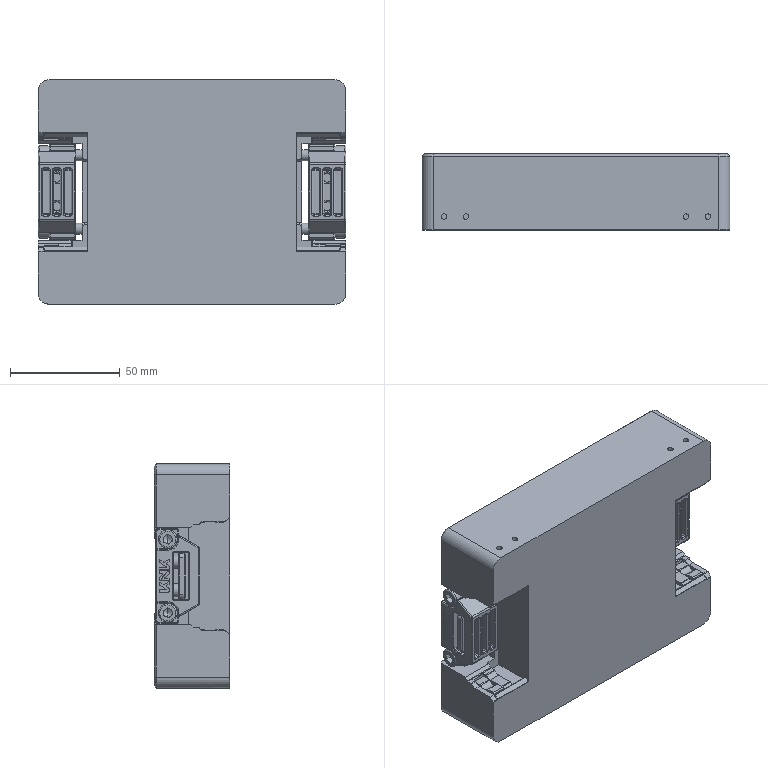Part | STEP file | Copy of K50-4 wheel slider (type B)^K50A-1H20-S(formula driven)-L300-motor left- | 1 solid | 1198 faces | box 140 x 34.5 x 102 mm | volume 434143 mm3 | plane 459 | cylinder 395 | spline 296 | cone 48 | commonest cylinder face diameters 1 x207 5 x44 0.4 x20 2 x20 0.98 x16 2.5 x16